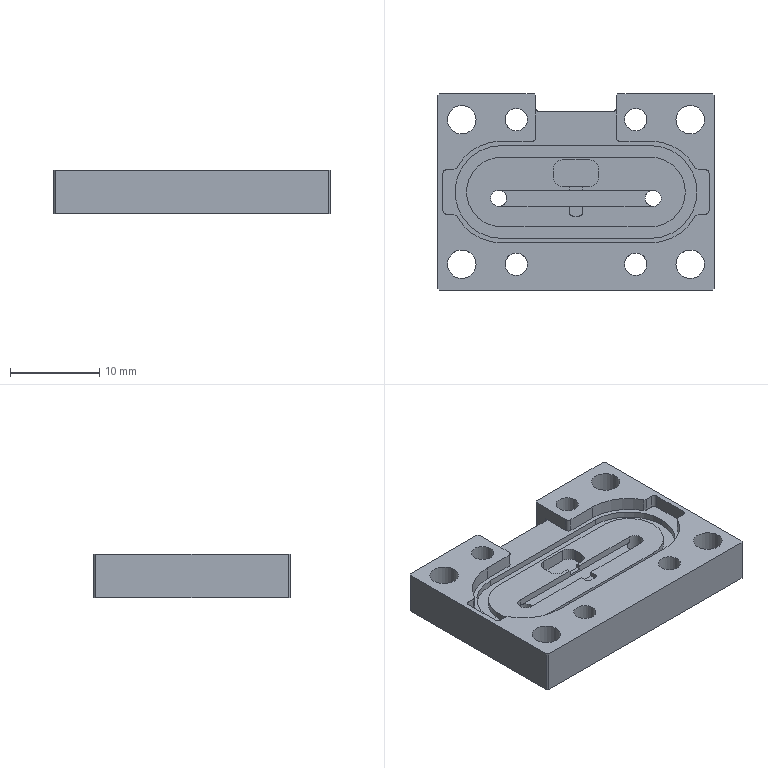NC program | NX | posted with a generic post | part box 31 x 22 x 4.9 mm
Lines 1661 to 2752 of 7945:
(PLANAR_MILL_4 , TOOL : 1.5C-4L-15L)
N3236 T04 M6
N3238 G54
N3240 G17 G0 G90 X-12.282 Y1.805 S3500 M3
N3242 G43 Z20. H4
N3244 Z0.14
N3246 G94 G1 Z-0.06 F500.
N3248 G3 X-12.968 Y1.976 R0.5
N3250 G1 X-13.251 Y1.806
N3252 G2 X-13.669 Y1.69 R0.81
N3254 G1 X-14.09
N3256 Y-1.69
N3258 X-13.669
N3260 G2 X-13.251 Y-1.806 R0.81
N3262 G1 X-12.968 Y-1.976
N3264 G3 X-12.282 Y-1.805 R0.5
N3266 G1 Z0.14
N3268 G0 Y1.805 Z0.08
N3270 G1 Z-0.12
N3272 G3 X-12.968 Y1.976 R0.5
N3274 G1 X-13.251 Y1.806
N3276 G2 X-13.669 Y1.69 R0.81
N3278 G1 X-14.09
N3280 Y-1.69
N3282 X-13.669
N3284 G2 X-13.251 Y-1.806 R0.81
N3286 G1 X-12.968 Y-1.976
N3288 G3 X-12.282 Y-1.805 R0.5
N3290 G1 Z0.08
N3292 G0 Y1.805 Z0.02
N3294 G1 Z-0.18
N3296 G3 X-12.968 Y1.976 R0.5
N3298 G1 X-13.251 Y1.806
N3300 G2 X-13.669 Y1.69 R0.81
N3302 G1 X-14.09
N3304 Y-1.69
N3306 X-13.669
N3308 G2 X-13.251 Y-1.806 R0.81
N3310 G1 X-12.968 Y-1.976
N3312 G3 X-12.282 Y-1.805 R0.5
N3314 G1 Z0.02
N3316 G0 Y1.805 Z-0.04
N3318 G1 Z-0.24
N3320 G3 X-12.968 Y1.976 R0.5
N3322 G1 X-13.251 Y1.806
N3324 G2 X-13.669 Y1.69 R0.81
N3326 G1 X-14.09
N3328 Y-1.69
N3330 X-13.669
N3332 G2 X-13.251 Y-1.806 R0.81
N3334 G1 X-12.968 Y-1.976
N3336 G3 X-12.282 Y-1.805 R0.5
N3338 G1 Z-0.04
N3340 G0 Y1.805 Z-0.1
N3342 G1 Z-0.3
N3344 G3 X-12.968 Y1.976 R0.5
N3346 G1 X-13.251 Y1.806
N3348 G2 X-13.669 Y1.69 R0.81
N3350 G1 X-14.09
N3352 Y-1.69
N3354 X-13.669
N3356 G2 X-13.251 Y-1.806 R0.81
N3358 G1 X-12.968 Y-1.976
N3360 G3 X-12.282 Y-1.805 R0.5
N3362 G1 Z-0.1
N3364 G0 Y1.805 Z-0.16
N3366 G1 Z-0.36
N3368 G3 X-12.968 Y1.976 R0.5
N3370 G1 X-13.251 Y1.806
N3372 G2 X-13.669 Y1.69 R0.81
N3374 G1 X-14.09
N3376 Y-1.69
N3378 X-13.669
N3380 G2 X-13.251 Y-1.806 R0.81
N3382 G1 X-12.968 Y-1.976
N3384 G3 X-12.282 Y-1.805 R0.5
N3386 G1 Z-0.16
N3388 G0 Y1.805 Z-0.22
N3390 G1 Z-0.42
N3392 G3 X-12.968 Y1.976 R0.5
N3394 G1 X-13.251 Y1.806
N3396 G2 X-13.669 Y1.69 R0.81
N3398 G1 X-14.09
N3400 Y-1.69
N3402 X-13.669
N3404 G2 X-13.251 Y-1.806 R0.81
N3406 G1 X-12.968 Y-1.976
N3408 G3 X-12.282 Y-1.805 R0.5
N3410 G1 Z-0.22
N3412 G0 Y1.805 Z-0.28
N3414 G1 Z-0.48
N3416 G3 X-12.968 Y1.976 R0.5
N3418 G1 X-13.251 Y1.806
N3420 G2 X-13.669 Y1.69 R0.81
N3422 G1 X-14.09
N3424 Y-1.69
N3426 X-13.669
N3428 G2 X-13.251 Y-1.806 R0.81
N3430 G1 X-12.968 Y-1.976
N3432 G3 X-12.282 Y-1.805 R0.5
N3434 G1 Z-0.28
N3436 G0 Y1.805 Z-0.34
N3438 G1 Z-0.54
N3440 G3 X-12.968 Y1.976 R0.5
N3442 G1 X-13.251 Y1.806
N3444 G2 X-13.669 Y1.69 R0.81
N3446 G1 X-14.09
N3448 Y-1.69
N3450 X-13.669
N3452 G2 X-13.251 Y-1.806 R0.81
N3454 G1 X-12.968 Y-1.976
N3456 G3 X-12.282 Y-1.805 R0.5
N3458 G1 Z-0.34
N3460 G0 Y1.805 Z-0.4
N3462 G1 Z-0.6
N3464 G3 X-12.968 Y1.976 R0.5
N3466 G1 X-13.251 Y1.806
N3468 G2 X-13.669 Y1.69 R0.81
N3470 G1 X-14.09
N3472 Y-1.69
N3474 X-13.669
N3476 G2 X-13.251 Y-1.806 R0.81
N3478 G1 X-12.968 Y-1.976
N3480 G3 X-12.282 Y-1.805 R0.5
N3482 G1 Z-0.4
N3484 G0 Y1.805 Z-0.46
N3486 G1 Z-0.66
N3488 G3 X-12.968 Y1.976 R0.5
N3490 G1 X-13.251 Y1.806
N3492 G2 X-13.669 Y1.69 R0.81
N3494 G1 X-14.09
N3496 Y-1.69
N3498 X-13.669
N3500 G2 X-13.251 Y-1.806 R0.81
N3502 G1 X-12.968 Y-1.976
N3504 G3 X-12.282 Y-1.805 R0.5
N3506 G1 Z-0.46
N3508 G0 Y1.805 Z-0.52
N3510 G1 Z-0.72
N3512 G3 X-12.968 Y1.976 R0.5
N3514 G1 X-13.251 Y1.806
N3516 G2 X-13.669 Y1.69 R0.81
N3518 G1 X-14.09
N3520 Y-1.69
N3522 X-13.669
N3524 G2 X-13.251 Y-1.806 R0.81
N3526 G1 X-12.968 Y-1.976
N3528 G3 X-12.282 Y-1.805 R0.5
N3530 G1 Z-0.52
N3532 G0 Y1.805 Z-0.58
N3534 G1 Z-0.78
N3536 G3 X-12.968 Y1.976 R0.5
N3538 G1 X-13.251 Y1.806
N3540 G2 X-13.669 Y1.69 R0.81
N3542 G1 X-14.09
N3544 Y-1.69
N3546 X-13.669
N3548 G2 X-13.251 Y-1.806 R0.81
N3550 G1 X-12.968 Y-1.976
N3552 G3 X-12.282 Y-1.805 R0.5
N3554 G1 Z-0.58
N3556 G0 Y1.805 Z-0.64
N3558 G1 Z-0.84
N3560 G3 X-12.968 Y1.976 R0.5
N3562 G1 X-13.251 Y1.806
N3564 G2 X-13.669 Y1.69 R0.81
N3566 G1 X-14.09
N3568 Y-1.69
N3570 X-13.669
N3572 G2 X-13.251 Y-1.806 R0.81
N3574 G1 X-12.968 Y-1.976
N3576 G3 X-12.282 Y-1.805 R0.5
N3578 G1 Z-0.64
N3580 G0 Y1.805 Z-0.7
N3582 G1 Z-0.9
N3584 G3 X-12.968 Y1.976 R0.5
N3586 G1 X-13.251 Y1.806
N3588 G2 X-13.669 Y1.69 R0.81
N3590 G1 X-14.09
N3592 Y-1.69
N3594 X-13.669
N3596 G2 X-13.251 Y-1.806 R0.81
N3598 G1 X-12.968 Y-1.976
N3600 G3 X-12.282 Y-1.805 R0.5
N3602 G1 Z-0.7
N3604 G0 Y1.805 Z-0.76
N3606 G1 Z-0.96
N3608 G3 X-12.968 Y1.976 R0.5
N3610 G1 X-13.251 Y1.806
N3612 G2 X-13.669 Y1.69 R0.81
N3614 G1 X-14.09
N3616 Y-1.69
N3618 X-13.669
N3620 G2 X-13.251 Y-1.806 R0.81
N3622 G1 X-12.968 Y-1.976
N3624 G3 X-12.282 Y-1.805 R0.5
N3626 G1 Z-0.76
N3628 G0 Y1.805 Z-0.82
N3630 G1 Z-1.02
N3632 G3 X-12.968 Y1.976 R0.5
N3634 G1 X-13.251 Y1.806
N3636 G2 X-13.669 Y1.69 R0.81
N3638 G1 X-14.09
N3640 Y-1.69
N3642 X-13.669
N3644 G2 X-13.251 Y-1.806 R0.81
N3646 G1 X-12.968 Y-1.976
N3648 G3 X-12.282 Y-1.805 R0.5
N3650 G1 Z-0.82
N3652 G0 Y1.805 Z-0.88
N3654 G1 Z-1.08
N3656 G3 X-12.968 Y1.976 R0.5
N3658 G1 X-13.251 Y1.806
N3660 G2 X-13.669 Y1.69 R0.81
N3662 G1 X-14.09
N3664 Y-1.69
N3666 X-13.669
N3668 G2 X-13.251 Y-1.806 R0.81
N3670 G1 X-12.968 Y-1.976
N3672 G3 X-12.282 Y-1.805 R0.5
N3674 G1 Z-0.88
N3676 G0 Y1.805 Z-0.94
N3678 G1 Z-1.14
N3680 G3 X-12.968 Y1.976 R0.5
N3682 G1 X-13.251 Y1.806
N3684 G2 X-13.669 Y1.69 R0.81
N3686 G1 X-14.09
N3688 Y-1.69
N3690 X-13.669
N3692 G2 X-13.251 Y-1.806 R0.81
N3694 G1 X-12.968 Y-1.976
N3696 G3 X-12.282 Y-1.805 R0.5
N3698 G1 Z-0.94
N3700 G0 Y1.805 Z-1.
N3702 G1 Z-1.2
N3704 G3 X-12.968 Y1.976 R0.5
N3706 G1 X-13.251 Y1.806
N3708 G2 X-13.669 Y1.69 R0.81
N3710 G1 X-14.09
N3712 Y-1.69
N3714 X-13.669
N3716 G2 X-13.251 Y-1.806 R0.81
N3718 G1 X-12.968 Y-1.976
N3720 G3 X-12.282 Y-1.805 R0.5
N3722 G1 Z-1.
N3724 G0 Y1.805 Z-1.06
N3726 G1 Z-1.26
N3728 G3 X-12.968 Y1.976 R0.5
N3730 G1 X-13.251 Y1.806
N3732 G2 X-13.669 Y1.69 R0.81
N3734 G1 X-14.09
N3736 Y-1.69
N3738 X-13.669
N3740 G2 X-13.251 Y-1.806 R0.81
N3742 G1 X-12.968 Y-1.976
N3744 G3 X-12.282 Y-1.805 R0.5
N3746 G1 Z-1.06
N3748 G0 Y1.805 Z-1.12
N3750 G1 Z-1.32
N3752 G3 X-12.968 Y1.976 R0.5
N3754 G1 X-13.251 Y1.806
N3756 G2 X-13.669 Y1.69 R0.81
N3758 G1 X-14.09
N3760 Y-1.69
N3762 X-13.669
N3764 G2 X-13.251 Y-1.806 R0.81
N3766 G1 X-12.968 Y-1.976
N3768 G3 X-12.282 Y-1.805 R0.5
N3770 G1 Z-1.12
N3772 G0 Y1.805 Z-1.18
N3774 G1 Z-1.38
N3776 G3 X-12.968 Y1.976 R0.5
N3778 G1 X-13.251 Y1.806
N3780 G2 X-13.669 Y1.69 R0.81
N3782 G1 X-14.09
N3784 Y-1.69
N3786 X-13.669
N3788 G2 X-13.251 Y-1.806 R0.81
N3790 G1 X-12.968 Y-1.976
N3792 G3 X-12.282 Y-1.805 R0.5
N3794 G1 Z-1.18
N3796 G0 Y1.805 Z-1.24
N3798 G1 Z-1.44
N3800 G3 X-12.968 Y1.976 R0.5
N3802 G1 X-13.251 Y1.806
N3804 G2 X-13.669 Y1.69 R0.81
N3806 G1 X-14.09
N3808 Y-1.69
N3810 X-13.669
N3812 G2 X-13.251 Y-1.806 R0.81
N3814 G1 X-12.968 Y-1.976
N3816 G3 X-12.282 Y-1.805 R0.5
N3818 G1 Z-1.24
N3820 G0 Y1.805 Z-1.25
N3822 G1 Z-1.45
N3824 G3 X-12.968 Y1.976 R0.5
N3826 G1 X-13.251 Y1.806
N3828 G2 X-13.669 Y1.69 R0.81
N3830 G1 X-14.09
N3832 Y-1.69
N3834 X-13.669
N3836 G2 X-13.251 Y-1.806 R0.81
N3838 G1 X-12.968 Y-1.976
N3840 G3 X-12.282 Y-1.805 R0.5
N3842 G1 Z-1.25
N3844 G0 Z3.
N3846 X12.282
N3848 Z0.14
N3850 G1 Z-0.06
N3852 G3 X12.968 Y-1.976 R0.5
N3854 G1 X13.251 Y-1.806
N3856 G2 X13.669 Y-1.69 R0.81
N3858 G1 X14.09
N3860 Y1.69
N3862 X13.669
N3864 G2 X13.251 Y1.806 R0.81
N3866 G1 X12.968 Y1.976
N3868 G3 X12.282 Y1.805 R0.5
N3870 G1 Z0.14
N3872 G0 Y-1.805 Z0.08
N3874 G1 Z-0.12
N3876 G3 X12.968 Y-1.976 R0.5
N3878 G1 X13.251 Y-1.806
N3880 G2 X13.669 Y-1.69 R0.81
N3882 G1 X14.09
N3884 Y1.69
N3886 X13.669
N3888 G2 X13.251 Y1.806 R0.81
N3890 G1 X12.968 Y1.976
N3892 G3 X12.282 Y1.805 R0.5
N3894 G1 Z0.08
N3896 G0 Y-1.805 Z0.02
N3898 G1 Z-0.18
N3900 G3 X12.968 Y-1.976 R0.5
N3902 G1 X13.251 Y-1.806
N3904 G2 X13.669 Y-1.69 R0.81
N3906 G1 X14.09
N3908 Y1.69
N3910 X13.669
N3912 G2 X13.251 Y1.806 R0.81
N3914 G1 X12.968 Y1.976
N3916 G3 X12.282 Y1.805 R0.5
N3918 G1 Z0.02
N3920 G0 Y-1.805 Z-0.04
N3922 G1 Z-0.24
N3924 G3 X12.968 Y-1.976 R0.5
N3926 G1 X13.251 Y-1.806
N3928 G2 X13.669 Y-1.69 R0.81
N3930 G1 X14.09
N3932 Y1.69
N3934 X13.669
N3936 G2 X13.251 Y1.806 R0.81
N3938 G1 X12.968 Y1.976
N3940 G3 X12.282 Y1.805 R0.5
N3942 G1 Z-0.04
N3944 G0 Y-1.805 Z-0.1
N3946 G1 Z-0.3
N3948 G3 X12.968 Y-1.976 R0.5
N3950 G1 X13.251 Y-1.806
N3952 G2 X13.669 Y-1.69 R0.81
N3954 G1 X14.09
N3956 Y1.69
N3958 X13.669
N3960 G2 X13.251 Y1.806 R0.81
N3962 G1 X12.968 Y1.976
N3964 G3 X12.282 Y1.805 R0.5
N3966 G1 Z-0.1
N3968 G0 Y-1.805 Z-0.16
N3970 G1 Z-0.36
N3972 G3 X12.968 Y-1.976 R0.5
N3974 G1 X13.251 Y-1.806
N3976 G2 X13.669 Y-1.69 R0.81
N3978 G1 X14.09
N3980 Y1.69
N3982 X13.669
N3984 G2 X13.251 Y1.806 R0.81
N3986 G1 X12.968 Y1.976
N3988 G3 X12.282 Y1.805 R0.5
N3990 G1 Z-0.16
N3992 G0 Y-1.805 Z-0.22
N3994 G1 Z-0.42
N3996 G3 X12.968 Y-1.976 R0.5
N3998 G1 X13.251 Y-1.806
N4000 G2 X13.669 Y-1.69 R0.81
N4002 G1 X14.09
N4004 Y1.69
N4006 X13.669
N4008 G2 X13.251 Y1.806 R0.81
N4010 G1 X12.968 Y1.976
N4012 G3 X12.282 Y1.805 R0.5
N4014 G1 Z-0.22
N4016 G0 Y-1.805 Z-0.28
N4018 G1 Z-0.48
N4020 G3 X12.968 Y-1.976 R0.5
N4022 G1 X13.251 Y-1.806
N4024 G2 X13.669 Y-1.69 R0.81
N4026 G1 X14.09
N4028 Y1.69
N4030 X13.669
N4032 G2 X13.251 Y1.806 R0.81
N4034 G1 X12.968 Y1.976
N4036 G3 X12.282 Y1.805 R0.5
N4038 G1 Z-0.28
N4040 G0 Y-1.805 Z-0.34
N4042 G1 Z-0.54
N4044 G3 X12.968 Y-1.976 R0.5
N4046 G1 X13.251 Y-1.806
N4048 G2 X13.669 Y-1.69 R0.81
N4050 G1 X14.09
N4052 Y1.69
N4054 X13.669
N4056 G2 X13.251 Y1.806 R0.81
N4058 G1 X12.968 Y1.976
N4060 G3 X12.282 Y1.805 R0.5
N4062 G1 Z-0.34
N4064 G0 Y-1.805 Z-0.4
N4066 G1 Z-0.6
N4068 G3 X12.968 Y-1.976 R0.5
N4070 G1 X13.251 Y-1.806
N4072 G2 X13.669 Y-1.69 R0.81
N4074 G1 X14.09
N4076 Y1.69
N4078 X13.669
N4080 G2 X13.251 Y1.806 R0.81
N4082 G1 X12.968 Y1.976
N4084 G3 X12.282 Y1.805 R0.5
N4086 G1 Z-0.4
N4088 G0 Y-1.805 Z-0.46
N4090 G1 Z-0.66
N4092 G3 X12.968 Y-1.976 R0.5
N4094 G1 X13.251 Y-1.806
N4096 G2 X13.669 Y-1.69 R0.81
N4098 G1 X14.09
N4100 Y1.69
N4102 X13.669
N4104 G2 X13.251 Y1.806 R0.81
N4106 G1 X12.968 Y1.976
N4108 G3 X12.282 Y1.805 R0.5
N4110 G1 Z-0.46
N4112 G0 Y-1.805 Z-0.52
N4114 G1 Z-0.72
N4116 G3 X12.968 Y-1.976 R0.5
N4118 G1 X13.251 Y-1.806
N4120 G2 X13.669 Y-1.69 R0.81
N4122 G1 X14.09
N4124 Y1.69
N4126 X13.669
N4128 G2 X13.251 Y1.806 R0.81
N4130 G1 X12.968 Y1.976
N4132 G3 X12.282 Y1.805 R0.5
N4134 G1 Z-0.52
N4136 G0 Y-1.805 Z-0.58
N4138 G1 Z-0.78
N4140 G3 X12.968 Y-1.976 R0.5
N4142 G1 X13.251 Y-1.806
N4144 G2 X13.669 Y-1.69 R0.81
N4146 G1 X14.09
N4148 Y1.69
N4150 X13.669
N4152 G2 X13.251 Y1.806 R0.81
N4154 G1 X12.968 Y1.976
N4156 G3 X12.282 Y1.805 R0.5
N4158 G1 Z-0.58
N4160 G0 Y-1.805 Z-0.64
N4162 G1 Z-0.84
N4164 G3 X12.968 Y-1.976 R0.5
N4166 G1 X13.251 Y-1.806
N4168 G2 X13.669 Y-1.69 R0.81
N4170 G1 X14.09
N4172 Y1.69
N4174 X13.669
N4176 G2 X13.251 Y1.806 R0.81
N4178 G1 X12.968 Y1.976
N4180 G3 X12.282 Y1.805 R0.5
N4182 G1 Z-0.64
N4184 G0 Y-1.805 Z-0.7
N4186 G1 Z-0.9
N4188 G3 X12.968 Y-1.976 R0.5
N4190 G1 X13.251 Y-1.806
N4192 G2 X13.669 Y-1.69 R0.81
N4194 G1 X14.09
N4196 Y1.69
N4198 X13.669
N4200 G2 X13.251 Y1.806 R0.81
N4202 G1 X12.968 Y1.976
N4204 G3 X12.282 Y1.805 R0.5
N4206 G1 Z-0.7
N4208 G0 Y-1.805 Z-0.76
N4210 G1 Z-0.96
N4212 G3 X12.968 Y-1.976 R0.5
N4214 G1 X13.251 Y-1.806
N4216 G2 X13.669 Y-1.69 R0.81
N4218 G1 X14.09
N4220 Y1.69
N4222 X13.669
N4224 G2 X13.251 Y1.806 R0.81
N4226 G1 X12.968 Y1.976
N4228 G3 X12.282 Y1.805 R0.5
N4230 G1 Z-0.76
N4232 G0 Y-1.805 Z-0.82
N4234 G1 Z-1.02
N4236 G3 X12.968 Y-1.976 R0.5
N4238 G1 X13.251 Y-1.806
N4240 G2 X13.669 Y-1.69 R0.81
N4242 G1 X14.09
N4244 Y1.69
N4246 X13.669
N4248 G2 X13.251 Y1.806 R0.81
N4250 G1 X12.968 Y1.976
N4252 G3 X12.282 Y1.805 R0.5
N4254 G1 Z-0.82
N4256 G0 Y-1.805 Z-0.88
N4258 G1 Z-1.08
N4260 G3 X12.968 Y-1.976 R0.5
N4262 G1 X13.251 Y-1.806
N4264 G2 X13.669 Y-1.69 R0.81
N4266 G1 X14.09
N4268 Y1.69
N4270 X13.669
N4272 G2 X13.251 Y1.806 R0.81
N4274 G1 X12.968 Y1.976
N4276 G3 X12.282 Y1.805 R0.5
N4278 G1 Z-0.88
N4280 G0 Y-1.805 Z-0.94
N4282 G1 Z-1.14
N4284 G3 X12.968 Y-1.976 R0.5
N4286 G1 X13.251 Y-1.806
N4288 G2 X13.669 Y-1.69 R0.81
N4290 G1 X14.09
N4292 Y1.69
N4294 X13.669
N4296 G2 X13.251 Y1.806 R0.81
N4298 G1 X12.968 Y1.976
N4300 G3 X12.282 Y1.805 R0.5
N4302 G1 Z-0.94
N4304 G0 Y-1.805 Z-1.
N4306 G1 Z-1.2
N4308 G3 X12.968 Y-1.976 R0.5
N4310 G1 X13.251 Y-1.806
N4312 G2 X13.669 Y-1.69 R0.81
N4314 G1 X14.09
N4316 Y1.69
N4318 X13.669
N4320 G2 X13.251 Y1.806 R0.81
N4322 G1 X12.968 Y1.976
N4324 G3 X12.282 Y1.805 R0.5
N4326 G1 Z-1.
N4328 G0 Y-1.805 Z-1.06
N4330 G1 Z-1.26
N4332 G3 X12.968 Y-1.976 R0.5
N4334 G1 X13.251 Y-1.806
N4336 G2 X13.669 Y-1.69 R0.81
N4338 G1 X14.09
N4340 Y1.69
N4342 X13.669
N4344 G2 X13.251 Y1.806 R0.81
N4346 G1 X12.968 Y1.976
N4348 G3 X12.282 Y1.805 R0.5
N4350 G1 Z-1.06
N4352 G0 Y-1.805 Z-1.12
N4354 G1 Z-1.32
N4356 G3 X12.968 Y-1.976 R0.5
N4358 G1 X13.251 Y-1.806
N4360 G2 X13.669 Y-1.69 R0.81
N4362 G1 X14.09
N4364 Y1.69
N4366 X13.669
N4368 G2 X13.251 Y1.806 R0.81
N4370 G1 X12.968 Y1.976
N4372 G3 X12.282 Y1.805 R0.5
N4374 G1 Z-1.12
N4376 G0 Y-1.805 Z-1.18
N4378 G1 Z-1.38
N4380 G3 X12.968 Y-1.976 R0.5
N4382 G1 X13.251 Y-1.806
N4384 G2 X13.669 Y-1.69 R0.81
N4386 G1 X14.09
N4388 Y1.69
N4390 X13.669
N4392 G2 X13.251 Y1.806 R0.81
N4394 G1 X12.968 Y1.976
N4396 G3 X12.282 Y1.805 R0.5
N4398 G1 Z-1.18
N4400 G0 Y-1.805 Z-1.24
N4402 G1 Z-1.44
N4404 G3 X12.968 Y-1.976 R0.5
N4406 G1 X13.251 Y-1.806
N4408 G2 X13.669 Y-1.69 R0.81
N4410 G1 X14.09
N4412 Y1.69
N4414 X13.669
N4416 G2 X13.251 Y1.806 R0.81
N4418 G1 X12.968 Y1.976
N4420 G3 X12.282 Y1.805 R0.5
N4422 G1 Z-1.24
N4424 G0 Y-1.805 Z-1.25
N4426 G1 Z-1.45
N4428 G3 X12.968 Y-1.976 R0.5
N4430 G1 X13.251 Y-1.806
N4432 G2 X13.669 Y-1.69 R0.81
N4434 G1 X14.09
N4436 Y1.69
N4438 X13.669
N4440 G2 X13.251 Y1.806 R0.81
N4442 G1 X12.968 Y1.976
N4444 G3 X12.282 Y1.805 R0.5
N4446 G1 Z-1.25
N4448 G0 Z20.
(PLANAR_MILL_4_COPY , TOOL : 1.5C-4L-15L)
N4450 X-4.127 Y12.28
N4452 Z0.14
N4454 G1 Z-0.06
N4456 G3 X-4.127 Y11.573 R0.5
N4458 G1 X-3.927 Y11.373
N4460 G2 X-3.69 Y10.8 R0.81
N4462 G1 Y9.81
N4464 X3.69
N4466 Y10.8
N4468 G2 X3.927 Y11.373 R0.81
N4470 G1 X4.127 Y11.573
N4472 G3 X4.127 Y12.28 R0.5
N4474 G1 Z0.14
N4476 G0 X-4.127 Z0.08
N4478 G1 Z-0.12
N4480 G3 X-4.127 Y11.573 R0.5
N4482 G1 X-3.927 Y11.373
N4484 G2 X-3.69 Y10.8 R0.81
N4486 G1 Y9.81
N4488 X3.69
N4490 Y10.8
N4492 G2 X3.927 Y11.373 R0.81
N4494 G1 X4.127 Y11.573
N4496 G3 X4.127 Y12.28 R0.5
N4498 G1 Z0.08
N4500 G0 X-4.127 Z0.02
N4502 G1 Z-0.18
N4504 G3 X-4.127 Y11.573 R0.5
N4506 G1 X-3.927 Y11.373
N4508 G2 X-3.69 Y10.8 R0.81
N4510 G1 Y9.81
N4512 X3.69
N4514 Y10.8
N4516 G2 X3.927 Y11.373 R0.81
N4518 G1 X4.127 Y11.573
N4520 G3 X4.127 Y12.28 R0.5
N4522 G1 Z0.02
N4524 G0 X-4.127 Z-0.04
N4526 G1 Z-0.24
N4528 G3 X-4.127 Y11.573 R0.5
N4530 G1 X-3.927 Y11.373
N4532 G2 X-3.69 Y10.8 R0.81
N4534 G1 Y9.81
N4536 X3.69
N4538 Y10.8
N4540 G2 X3.927 Y11.373 R0.81
N4542 G1 X4.127 Y11.573
N4544 G3 X4.127 Y12.28 R0.5
N4546 G1 Z-0.04
N4548 G0 X-4.127 Z-0.1
N4550 G1 Z-0.3
N4552 G3 X-4.127 Y11.573 R0.5
N4554 G1 X-3.927 Y11.373
N4556 G2 X-3.69 Y10.8 R0.81
N4558 G1 Y9.81
N4560 X3.69
N4562 Y10.8
N4564 G2 X3.927 Y11.373 R0.81
N4566 G1 X4.127 Y11.573
N4568 G3 X4.127 Y12.28 R0.5
N4570 G1 Z-0.1
N4572 G0 X-4.127 Z-0.16
N4574 G1 Z-0.36
N4576 G3 X-4.127 Y11.573 R0.5
N4578 G1 X-3.927 Y11.373
N4580 G2 X-3.69 Y10.8 R0.81
N4582 G1 Y9.81
N4584 X3.69
N4586 Y10.8
N4588 G2 X3.927 Y11.373 R0.81
N4590 G1 X4.127 Y11.573
N4592 G3 X4.127 Y12.28 R0.5
N4594 G1 Z-0.16
N4596 G0 X-4.127 Z-0.22
N4598 G1 Z-0.42
N4600 G3 X-4.127 Y11.573 R0.5
N4602 G1 X-3.927 Y11.373
N4604 G2 X-3.69 Y10.8 R0.81
N4606 G1 Y9.81
N4608 X3.69
N4610 Y10.8
N4612 G2 X3.927 Y11.373 R0.81
N4614 G1 X4.127 Y11.573
N4616 G3 X4.127 Y12.28 R0.5
N4618 G1 Z-0.22
N4620 G0 X-4.127 Z-0.28
N4622 G1 Z-0.48
N4624 G3 X-4.127 Y11.573 R0.5
N4626 G1 X-3.927 Y11.373
N4628 G2 X-3.69 Y10.8 R0.81
N4630 G1 Y9.81
N4632 X3.69
N4634 Y10.8
N4636 G2 X3.927 Y11.373 R0.81
N4638 G1 X4.127 Y11.573
N4640 G3 X4.127 Y12.28 R0.5
N4642 G1 Z-0.28
N4644 G0 X-4.127 Z-0.34
N4646 G1 Z-0.54
N4648 G3 X-4.127 Y11.573 R0.5
N4650 G1 X-3.927 Y11.373
N4652 G2 X-3.69 Y10.8 R0.81
N4654 G1 Y9.81
N4656 X3.69
N4658 Y10.8
N4660 G2 X3.927 Y11.373 R0.81
N4662 G1 X4.127 Y11.573
N4664 G3 X4.127 Y12.28 R0.5
N4666 G1 Z-0.34
N4668 G0 X-4.127 Z-0.4
N4670 G1 Z-0.6
N4672 G3 X-4.127 Y11.573 R0.5
N4674 G1 X-3.927 Y11.373
N4676 G2 X-3.69 Y10.8 R0.81
N4678 G1 Y9.81
N4680 X3.69
N4682 Y10.8
N4684 G2 X3.927 Y11.373 R0.81
N4686 G1 X4.127 Y11.573
N4688 G3 X4.127 Y12.28 R0.5
N4690 G1 Z-0.4
N4692 G0 X-4.127 Z-0.46
N4694 G1 Z-0.66
N4696 G3 X-4.127 Y11.573 R0.5
N4698 G1 X-3.927 Y11.373
N4700 G2 X-3.69 Y10.8 R0.81
N4702 G1 Y9.81
N4704 X3.69
N4706 Y10.8
N4708 G2 X3.927 Y11.373 R0.81
N4710 G1 X4.127 Y11.573
N4712 G3 X4.127 Y12.28 R0.5
N4714 G1 Z-0.46
N4716 G0 X-4.127 Z-0.52
N4718 G1 Z-0.72
N4720 G3 X-4.127 Y11.573 R0.5
N4722 G1 X-3.927 Y11.373
N4724 G2 X-3.69 Y10.8 R0.81
N4726 G1 Y9.81
N4728 X3.69
N4730 Y10.8
N4732 G2 X3.927 Y11.373 R0.81
N4734 G1 X4.127 Y11.573
N4736 G3 X4.127 Y12.28 R0.5
N4738 G1 Z-0.52
N4740 G0 X-4.127 Z-0.58
N4742 G1 Z-0.78
N4744 G3 X-4.127 Y11.573 R0.5
N4746 G1 X-3.927 Y11.373
N4748 G2 X-3.69 Y10.8 R0.81
N4750 G1 Y9.81
N4752 X3.69
N4754 Y10.8
N4756 G2 X3.927 Y11.373 R0.81
N4758 G1 X4.127 Y11.573
N4760 G3 X4.127 Y12.28 R0.5
N4762 G1 Z-0.58
N4764 G0 X-4.127 Z-0.64
N4766 G1 Z-0.84
N4768 G3 X-4.127 Y11.573 R0.5
N4770 G1 X-3.927 Y11.373
N4772 G2 X-3.69 Y10.8 R0.81
N4774 G1 Y9.81
N4776 X3.69
N4778 Y10.8
N4780 G2 X3.927 Y11.373 R0.81
N4782 G1 X4.127 Y11.573
N4784 G3 X4.127 Y12.28 R0.5
N4786 G1 Z-0.64
N4788 G0 X-4.127 Z-0.7
N4790 G1 Z-0.9
N4792 G3 X-4.127 Y11.573 R0.5
N4794 G1 X-3.927 Y11.373
N4796 G2 X-3.69 Y10.8 R0.81
N4798 G1 Y9.81
N4800 X3.69
N4802 Y10.8
N4804 G2 X3.927 Y11.373 R0.81
N4806 G1 X4.127 Y11.573
N4808 G3 X4.127 Y12.28 R0.5
N4810 G1 Z-0.7
N4812 G0 X-4.127 Z-0.76
N4814 G1 Z-0.96
N4816 G3 X-4.127 Y11.573 R0.5
N4818 G1 X-3.927 Y11.373
N4820 G2 X-3.69 Y10.8 R0.81
N4822 G1 Y9.81
N4824 X3.69
N4826 Y10.8
N4828 G2 X3.927 Y11.373 R0.81
N4830 G1 X4.127 Y11.573
N4832 G3 X4.127 Y12.28 R0.5
N4834 G1 Z-0.76
N4836 G0 X-4.127 Z-0.82
N4838 G1 Z-1.02
N4840 G3 X-4.127 Y11.573 R0.5
N4842 G1 X-3.927 Y11.373
N4844 G2 X-3.69 Y10.8 R0.81
N4846 G1 Y9.81
N4848 X3.69
N4850 Y10.8
N4852 G2 X3.927 Y11.373 R0.81
N4854 G1 X4.127 Y11.573
N4856 G3 X4.127 Y12.28 R0.5
N4858 G1 Z-0.82
N4860 G0 X-4.127 Z-0.88
N4862 G1 Z-1.08
N4864 G3 X-4.127 Y11.573 R0.5
N4866 G1 X-3.927 Y11.373
N4868 G2 X-3.69 Y10.8 R0.81
N4870 G1 Y9.81
N4872 X3.69
N4874 Y10.8
N4876 G2 X3.927 Y11.373 R0.81
N4878 G1 X4.127 Y11.573
N4880 G3 X4.127 Y12.28 R0.5
N4882 G1 Z-0.88
N4884 G0 X-4.127 Z-0.94
N4886 G1 Z-1.14
N4888 G3 X-4.127 Y11.573 R0.5
N4890 G1 X-3.927 Y11.373
N4892 G2 X-3.69 Y10.8 R0.81
N4894 G1 Y9.81
N4896 X3.69
N4898 Y10.8
N4900 G2 X3.927 Y11.373 R0.81
N4902 G1 X4.127 Y11.573
N4904 G3 X4.127 Y12.28 R0.5
N4906 G1 Z-0.94
N4908 G0 X-4.127 Z-1.
N4910 G1 Z-1.2
N4912 G3 X-4.127 Y11.573 R0.5
N4914 G1 X-3.927 Y11.373
N4916 G2 X-3.69 Y10.8 R0.81
N4918 G1 Y9.81
N4920 X3.69
N4922 Y10.8
N4924 G2 X3.927 Y11.373 R0.81
N4926 G1 X4.127 Y11.573
N4928 G3 X4.127 Y12.28 R0.5
N4930 G1 Z-1.
N4932 G0 X-4.127 Z-1.06
N4934 G1 Z-1.26
N4936 G3 X-4.127 Y11.573 R0.5
N4938 G1 X-3.927 Y11.373
N4940 G2 X-3.69 Y10.8 R0.81
N4942 G1 Y9.81
N4944 X3.69
N4946 Y10.8
N4948 G2 X3.927 Y11.373 R0.81
N4950 G1 X4.127 Y11.573
N4952 G3 X4.127 Y12.28 R0.5
N4954 G1 Z-1.06
N4956 G0 X-4.127 Z-1.12
N4958 G1 Z-1.32
N4960 G3 X-4.127 Y11.573 R0.5
N4962 G1 X-3.927 Y11.373
N4964 G2 X-3.69 Y10.8 R0.81
N4966 G1 Y9.81
N4968 X3.69
N4970 Y10.8
N4972 G2 X3.927 Y11.373 R0.81
N4974 G1 X4.127 Y11.573
N4976 G3 X4.127 Y12.28 R0.5
N4978 G1 Z-1.12
N4980 G0 X-4.127 Z-1.18
N4982 G1 Z-1.38
N4984 G3 X-4.127 Y11.573 R0.5
N4986 G1 X-3.927 Y11.373
N4988 G2 X-3.69 Y10.8 R0.81
N4990 G1 Y9.81
N4992 X3.69
N4994 Y10.8
N4996 G2 X3.927 Y11.373 R0.81
N4998 G1 X4.127 Y11.573
N5000 G3 X4.127 Y12.28 R0.5
N5002 G1 Z-1.18
N5004 G0 X-4.127 Z-1.24
N5006 G1 Z-1.44
N5008 G3 X-4.127 Y11.573 R0.5
N5010 G1 X-3.927 Y11.373
N5012 G2 X-3.69 Y10.8 R0.81
N5014 G1 Y9.81
N5016 X3.69
N5018 Y10.8
N5020 G2 X3.927 Y11.373 R0.81
N5022 G1 X4.127 Y11.573
N5024 G3 X4.127 Y12.28 R0.5
N5026 G1 Z-1.24
N5028 G0 X-4.127 Z-1.3
N5030 G1 Z-1.5
N5032 G3 X-4.127 Y11.573 R0.5
N5034 G1 X-3.927 Y11.373
N5036 G2 X-3.69 Y10.8 R0.81
N5038 G1 Y9.81
N5040 X3.69
N5042 Y10.8
N5044 G2 X3.927 Y11.373 R0.81
N5046 G1 X4.127 Y11.573
N5048 G3 X4.127 Y12.28 R0.5
N5050 G1 Z-1.3
N5052 G0 X-4.127 Z-1.36
N5054 G1 Z-1.56
N5056 G3 X-4.127 Y11.573 R0.5
N5058 G1 X-3.927 Y11.373
N5060 G2 X-3.69 Y10.8 R0.81
N5062 G1 Y9.81
N5064 X3.69
N5066 Y10.8
N5068 G2 X3.927 Y11.373 R0.81
N5070 G1 X4.127 Y11.573
N5072 G3 X4.127 Y12.28 R0.5
N5074 G1 Z-1.36
N5076 G0 X-4.127 Z-1.42
N5078 G1 Z-1.62
N5080 G3 X-4.127 Y11.573 R0.5
N5082 G1 X-3.927 Y11.373
N5084 G2 X-3.69 Y10.8 R0.81
N5086 G1 Y9.81
N5088 X3.69
N5090 Y10.8
N5092 G2 X3.927 Y11.373 R0.81
N5094 G1 X4.127 Y11.573
N5096 G3 X4.127 Y12.28 R0.5
N5098 G1 Z-1.42
N5100 G0 X-4.127 Z-1.48
N5102 G1 Z-1.68
N5104 G3 X-4.127 Y11.573 R0.5
N5106 G1 X-3.927 Y11.373
N5108 G2 X-3.69 Y10.8 R0.81
N5110 G1 Y9.81
N5112 X3.69
N5114 Y10.8
N5116 G2 X3.927 Y11.373 R0.81
N5118 G1 X4.127 Y11.573
N5120 G3 X4.127 Y12.28 R0.5
N5122 G1 Z-1.48
N5124 G0 X-4.127 Z-1.54
N5126 G1 Z-1.74
N5128 G3 X-4.127 Y11.573 R0.5
N5130 G1 X-3.927 Y11.373
N5132 G2 X-3.69 Y10.8 R0.81
N5134 G1 Y9.81
N5136 X3.69
N5138 Y10.8
N5140 G2 X3.927 Y11.373 R0.81
N5142 G1 X4.127 Y11.573
N5144 G3 X4.127 Y12.28 R0.5
N5146 G1 Z-1.54
N5148 G0 X-4.127 Z-1.6
N5150 G1 Z-1.8
N5152 G3 X-4.127 Y11.573 R0.5
N5154 G1 X-3.927 Y11.373
N5156 G2 X-3.69 Y10.8 R0.81
N5158 G1 Y9.81
N5160 X3.69
N5162 Y10.8
N5164 G2 X3.927 Y11.373 R0.81
N5166 G1 X4.127 Y11.573
N5168 G3 X4.127 Y12.28 R0.5
N5170 G1 Z-1.6
N5172 G0 X-4.127 Z-1.66
N5174 G1 Z-1.86
N5176 G3 X-4.127 Y11.573 R0.5
N5178 G1 X-3.927 Y11.373
N5180 G2 X-3.69 Y10.8 R0.81
N5182 G1 Y9.81
N5184 X3.69
N5186 Y10.8
N5188 G2 X3.927 Y11.373 R0.81
N5190 G1 X4.127 Y11.573
N5192 G3 X4.127 Y12.28 R0.5
N5194 G1 Z-1.66
N5196 G0 X-4.127 Z-1.72
N5198 G1 Z-1.92
N5200 G3 X-4.127 Y11.573 R0.5
N5202 G1 X-3.927 Y11.373
N5204 G2 X-3.69 Y10.8 R0.81
N5206 G1 Y9.81
N5208 X3.69
N5210 Y10.8
N5212 G2 X3.927 Y11.373 R0.81
N5214 G1 X4.127 Y11.573
N5216 G3 X4.127 Y12.28 R0.5
N5218 G1 Z-1.72
N5220 G0 X-4.127 Z-1.78
N5222 G1 Z-1.98
N5224 G3 X-4.127 Y11.573 R0.5
N5226 G1 X-3.927 Y11.373
N5228 G2 X-3.69 Y10.8 R0.81
N5230 G1 Y9.81
N5232 X3.69
N5234 Y10.8
N5236 G2 X3.927 Y11.373 R0.81
N5238 G1 X4.127 Y11.573
N5240 G3 X4.127 Y12.28 R0.5
N5242 G1 Z-1.78
N5244 G0 X-4.127 Z-1.84
N5246 G1 Z-2.04
N5248 G3 X-4.127 Y11.573 R0.5
N5250 G1 X-3.927 Y11.373
N5252 G2 X-3.69 Y10.8 R0.81
N5254 G1 Y9.81
N5256 X3.69
N5258 Y10.8
N5260 G2 X3.927 Y11.373 R0.81
N5262 G1 X4.127 Y11.573
N5264 G3 X4.127 Y12.28 R0.5
N5266 G1 Z-1.84
N5268 G0 X-4.127 Z-1.9
N5270 G1 Z-2.1
N5272 G3 X-4.127 Y11.573 R0.5
N5274 G1 X-3.927 Y11.373
N5276 G2 X-3.69 Y10.8 R0.81
N5278 G1 Y9.81
N5280 X3.69
N5282 Y10.8
N5284 G2 X3.927 Y11.373 R0.81
N5286 G1 X4.127 Y11.573
N5288 G3 X4.127 Y12.28 R0.5
N5290 G1 Z-1.9
N5292 G0 X-4.127 Z-1.96
N5294 G1 Z-2.16
N5296 G3 X-4.127 Y11.573 R0.5
N5298 G1 X-3.927 Y11.373
N5300 G2 X-3.69 Y10.8 R0.81
N5302 G1 Y9.81
N5304 X3.69
N5306 Y10.8
N5308 G2 X3.927 Y11.373 R0.81
N5310 G1 X4.127 Y11.573
N5312 G3 X4.127 Y12.28 R0.5
N5314 G1 Z-1.96
N5316 G0 X-4.127 Z-2.02
N5318 G1 Z-2.22
N5320 G3 X-4.127 Y11.573 R0.5
N5322 G1 X-3.927 Y11.373
N5324 G2 X-3.69 Y10.8 R0.81
N5326 G1 Y9.81
N5328 X3.69
N5330 Y10.8
N5332 G2 X3.927 Y11.373 R0.81
N5334 G1 X4.127 Y11.573
N5336 G3 X4.127 Y12.28 R0.5
N5338 G1 Z-2.02
N5340 G0 X-4.127 Z-2.08
N5342 G1 Z-2.28
N5344 G3 X-4.127 Y11.573 R0.5
N5346 G1 X-3.927 Y11.373
N5348 G2 X-3.69 Y10.8 R0.81
N5350 G1 Y9.81
N5352 X3.69
N5354 Y10.8
N5356 G2 X3.927 Y11.373 R0.81
N5358 G1 X4.127 Y11.573
N5360 G3 X4.127 Y12.28 R0.5
N5362 G1 Z-2.08
N5364 G0 X-4.127 Z-2.14
N5366 G1 Z-2.34
N5368 G3 X-4.127 Y11.573 R0.5
N5370 G1 X-3.927 Y11.373
N5372 G2 X-3.69 Y10.8 R0.81
N5374 G1 Y9.81
N5376 X3.69
N5378 Y10.8
N5380 G2 X3.927 Y11.373 R0.81
N5382 G1 X4.127 Y11.573
N5384 G3 X4.127 Y12.28 R0.5
N5386 G1 Z-2.14
N5388 G0 X-4.127 Z-2.2
N5390 G1 Z-2.4
N5392 G3 X-4.127 Y11.573 R0.5
N5394 G1 X-3.927 Y11.373
N5396 G2 X-3.69 Y10.8 R0.81
N5398 G1 Y9.81
N5400 X3.69
N5402 Y10.8
N5404 G2 X3.927 Y11.373 R0.81
N5406 G1 X4.127 Y11.573